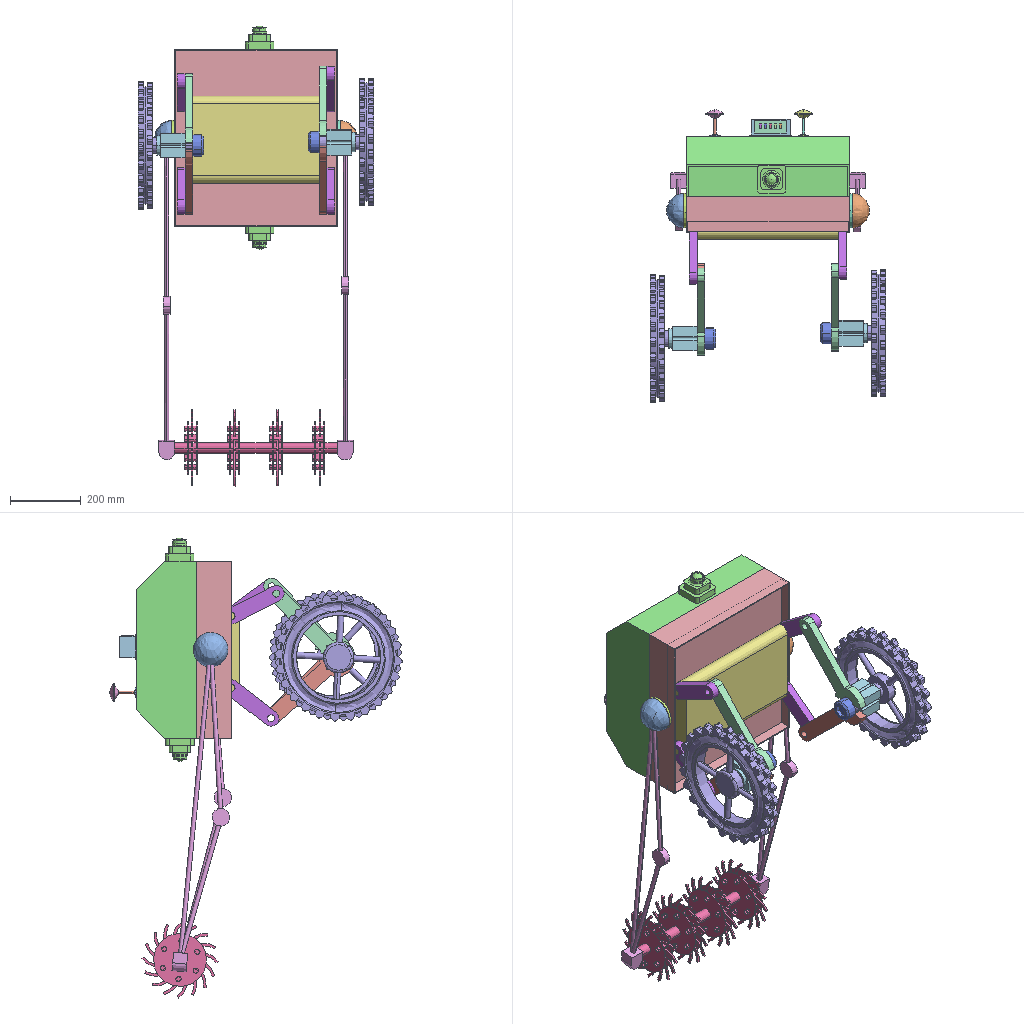Assembly | SolidWorks | 16 different items | 26 placed | box 663 x 825 x 1298 mm
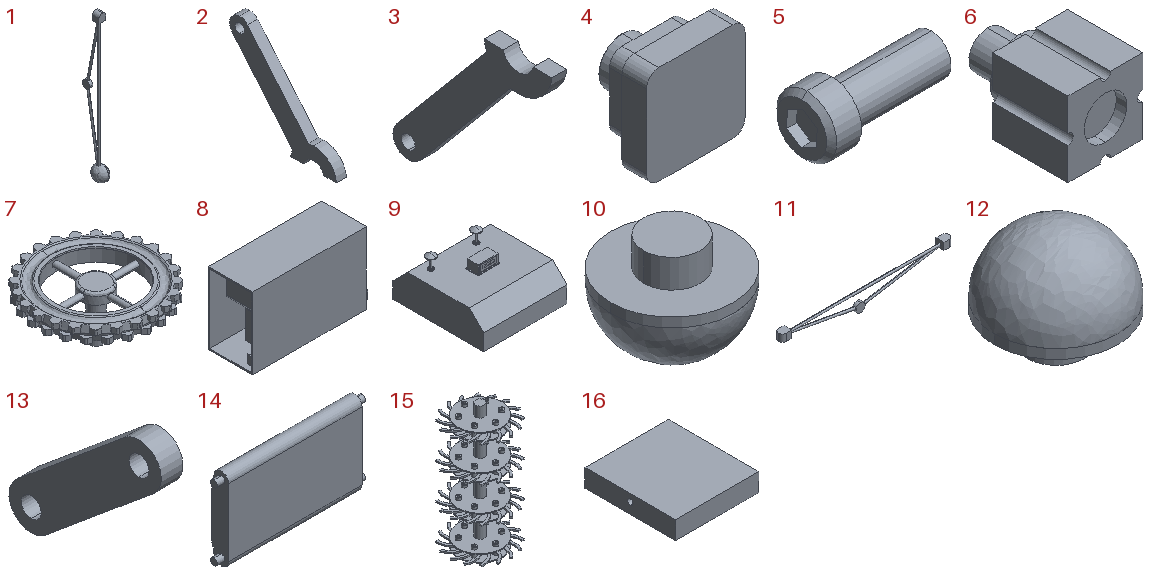Parts list (item | name | quantity | parent item | size | volume | features):
1 | (subassembly) | x1 | - | 78.75 x 149.147 x 960.154 mm | 541378 mm3 | features CompositeCurve 1
2 | - | x2 | - | 22 x 233.027 x 209.178 mm | 273312 mm3 | features BaseBody 14, ICE 7, MoveFace 2
3 | - | x2 | - | 22 x 233.027 x 209.178 mm | 273312 mm3 | features BaseBody 14, ICE 7, MoveFace 2
4 | - | x2 | - | 80 x 65.1 x 80 mm | 221973 mm3 | features ICE 5, Fillet 2, Dome 1, Extrusion 1
5 | - | x2 | - | 130 x 60 x 60 mm | 200467 mm3 | features BaseBody 12, ICE 10, Chamfer 2
6 | - | x2 | - | 70 x 110 x 70 mm | 372060 mm3 | features ICE 3, Extrusion 1
7 | - | x2 | - | 360.432 x 360.432 x 153.62 mm | 1936645 mm3 | features BaseBody 1, MoveFace 1, Scale 1
8 | - | x1 | - | 406 x 155 x 251.525 mm | 5535552 mm3 | features BaseBody 5
9 | - | x1 | - | 460 x 500 x 244.744 mm | 2933246 mm3 | features BaseBody 16, Chamfer 1
10 | - | x1 | - | 97.5 x 97.5 x 78.75 mm | 152963 mm3 | features BaseBody 2, ICE 1, Scale 1
11 | - | x2 | in 1 | 944 x 44 x 120.397 mm | 388537 mm3 | features MoveFace 4, BaseBody 2, Sweep 1
12 | - | x1 | in 1 | 97.5 x 97.5 x 78.75 mm | 152792 mm3 | features BaseBody 2, ICE 1, Scale 1
13 | - | x4 | - | 22 x 153.344 x 135.399 mm | 160860 mm3 | features BaseBody 1, ICE 1, MoveFace 1
14 | - | x1 | - | 444 x 50.745 x 246.557 mm | 4628488 mm3 | features BaseBody 11, ICE 10, Chamfer 2
15 | - | x1 | - | 214.882 x 214.882 x 460 mm | 1059862 mm3 | features BaseBody 12, MoveFace 3, ICE 2, Scale 1
16 | - | x1 | - | 460 x 500 x 100 mm | 15946565 mm3 | features BaseBody 1, ICE 1
Mates (type | each side: item.copy, entity, surface, feature):
In the top assembly
Concentric | 10.1 face cylinder Cut-Extrude1 | 11.1 select_type:24
Coincident | 10.1 face plane Input 1 | 11.1 face plane Input 3
Concentric | 16.1 face cylinder Cut-Extrude2 | 10.1 face cylinder Cut-Extrude1
Coincident | 16.1 face plane Input 1 | 10.1 face plane Input 1
Coincident | 9.1 face plane Input 8 | 4.1 face plane Boss-Extrude1
DistanceDim | 4.1 face plane Boss-Extrude1 | 9.1 face plane Input 8
Coincident | 9.1 face plane Input 8 | 4.2 face plane Boss-Extrude1
DistanceDim | 4.2 face plane Boss-Extrude1 | 9.1 face plane Input 8
Concentric | 16.1 face cylinder Cut-Extrude2 | 12.1 face cylinder Cut-Extrude1
Coincident | 16.1 face plane Input 1 | 12.1 face plane Input 2
Coincident | 11.2 face plane Input 3 | 11.1 face plane Input 3
Concentric | 11.2 select_type:24 | 15.1 face cylinder Boss-Extrude2
Coincident | 11.2 face plane Input 3 | 15.1 face plane Boss-Extrude2
Concentric | 7.1 face cylinder Input 1 | 6.1 face cylinder Cut-Extrude1
Concentric | 7.2 face cylinder Input 1 | 6.2 face cylinder Boss-Extrude3
Coincident | 16.1 face plane Input 1 | 14.1 face plane Input 3
DistanceDim | 16.1 face plane Input 1 | 14.1 face plane Boss-Extrude9
Concentric | 14.1 face cylinder Boss-Extrude9 | 13.1 face cylinder Cut-Extrude1
Coincident | 14.1 face plane Input 3 | 13.1 face plane Input 11
Concentric | 14.1 face cylinder Boss-Extrude9 | 13.2 face cylinder Cut-Extrude1
Coincident | 14.1 face plane Input 3 | 13.2 face plane Input 11
Concentric | 14.1 face cylinder Boss-Extrude10 | 13.3 face cylinder Cut-Extrude1
Concentric | 14.1 face cylinder Boss-Extrude10 | 13.4 face cylinder Cut-Extrude1
Coincident | 14.1 face plane Input 3 | 13.4 face plane Input 11
Coincident | 14.1 face plane Input 3 | 13.3 face plane Input 11
Concentric | 13.1 face cylinder Cut-Extrude1 | 2.1 face cylinder Cut-Extrude9
Coincident | 13.1 face plane Input 11 | 2.1 face plane Input 5
Concentric | 13.2 face cylinder Cut-Extrude1 | 3.1 face cylinder Cut-Extrude9
Coincident | 13.2 face plane Input 11 | 3.1 face plane Input 5
Concentric | 13.4 face cylinder Cut-Extrude1 | 2.2 face cylinder Cut-Extrude9
Coincident | 13.4 face plane Input 11 | 2.2 face plane Input 5
Concentric | 13.3 face cylinder Cut-Extrude1 | 3.2 face cylinder Cut-Extrude9
Coincident | 13.3 face plane Input 11 | 3.2 face plane Input 5
Coincident | 6.1 face plane Boss-Extrude1 | 3.1 face plane Input 5
Coincident | 6.2 face plane Boss-Extrude1 | 2.2 face plane Input 5
Coincident | 7.2 face plane Input 1 | 3.2 face plane Input 5
Coincident | 7.1 face plane Input 1 | 2.1 face plane Input 5
Coincident | 3.1 face plane Input 5 | 5.1 face plane Boss-Extrude7
Coincident | 3.2 face plane Input 5 | 5.2 face plane Boss-Extrude7 | 2 times
Concentric | 7.1 face cylinder Input 1 | 5.1 face cylinder Boss-Extrude7
Concentric | 7.2 face cylinder Input 1 | 5.2 face cylinder Boss-Extrude7
In subassembly 1
Coincident | 12.2 face plane Input 2 | 11.1 face plane Input 3
Concentric | 12.2 face cylinder Cut-Extrude1 | 11.1 select_type:24